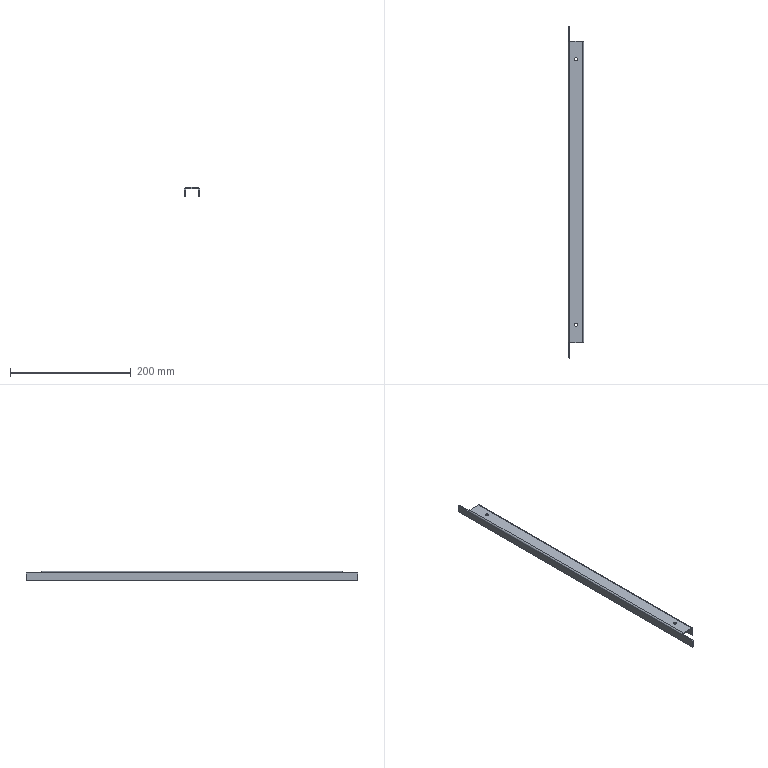Part | STEP file | Clamp Frame Weldment 2 | 1 solid | 22 faces | box 25 x 550 x 15 mm | volume 50877 mm3 | plane 14 | cylinder 8 | commonest cylinder face diameters 5.2 x4 1 x2 5 x2
STEP:
#1=CARTESIAN_POINT('',(-534.9,391.433,-2.));
#2=VERTEX_POINT('',#1);
#3=CARTESIAN_POINT('',(-540.1,391.433,-2.));
#4=VERTEX_POINT('',#3);
#5=CARTESIAN_POINT('',(-537.5,391.433,-2.));
#6=DIRECTION('',(0.,0.,-1.));
#7=DIRECTION('',(1.,0.,0.));
#8=AXIS2_PLACEMENT_3D('',#5,#6,#7);
#9=CIRCLE('',#8,2.6);
#10=EDGE_CURVE('',#2,#4,#9,.T.);
#11=ORIENTED_EDGE('',*,*,#10,.T.);
#12=CARTESIAN_POINT('',(-540.1,391.433,0.));
#13=VERTEX_POINT('',#12);
#14=CARTESIAN_POINT('',(-540.1,391.433,-10.));
#15=DIRECTION('',(0.,0.,1.));
#16=VECTOR('',#15,1000.);
#17=LINE('',#14,#16);
#18=EDGE_CURVE('',#4,#13,#17,.T.);
#19=ORIENTED_EDGE('',*,*,#18,.T.);
#20=CARTESIAN_POINT('',(-534.9,391.433,0.));
#21=VERTEX_POINT('',#20);
#22=CARTESIAN_POINT('',(-537.5,391.433,0.));
#23=DIRECTION('',(0.,0.,-1.));
#24=DIRECTION('',(1.,0.,0.));
#25=AXIS2_PLACEMENT_3D('',#22,#23,#24);
#26=CIRCLE('',#25,2.6);
#27=EDGE_CURVE('',#21,#13,#26,.T.);
#28=ORIENTED_EDGE('',*,*,#27,.F.);
#29=CARTESIAN_POINT('',(-534.9,391.433,-10.));
#30=DIRECTION('',(0.,0.,1.));
#31=VECTOR('',#30,1000.);
#32=LINE('',#29,#31);
#33=EDGE_CURVE('',#2,#21,#32,.T.);
#34=ORIENTED_EDGE('',*,*,#33,.F.);
#35=EDGE_LOOP('',(#11,#19,#28,#34));
#36=FACE_OUTER_BOUND('',#35,.T.);
#37=CARTESIAN_POINT('',(-537.5,391.433,-10.));
#38=DIRECTION('',(0.,0.,1.));
#39=DIRECTION('',(1.,0.,0.));
#40=AXIS2_PLACEMENT_3D('',#37,#38,#39);
#41=CYLINDRICAL_SURFACE('',#40,2.6);
#42=ADVANCED_FACE('',(#36),#41,.F.);
#43=CARTESIAN_POINT('',(-534.9,831.433,-2.));
#44=VERTEX_POINT('',#43);
#45=CARTESIAN_POINT('',(-540.1,831.433,-2.));
#46=VERTEX_POINT('',#45);
#47=CARTESIAN_POINT('',(-537.5,831.433,-2.));
#48=DIRECTION('',(0.,0.,-1.));
#49=DIRECTION('',(1.,0.,0.));
#50=AXIS2_PLACEMENT_3D('',#47,#48,#49);
#51=CIRCLE('',#50,2.6);
#52=EDGE_CURVE('',#44,#46,#51,.T.);
#53=ORIENTED_EDGE('',*,*,#52,.T.);
#54=CARTESIAN_POINT('',(-540.1,831.433,0.));
#55=VERTEX_POINT('',#54);
#56=CARTESIAN_POINT('',(-540.1,831.433,-10.));
#57=DIRECTION('',(0.,0.,1.));
#58=VECTOR('',#57,1000.);
#59=LINE('',#56,#58);
#60=EDGE_CURVE('',#46,#55,#59,.T.);
#61=ORIENTED_EDGE('',*,*,#60,.T.);
#62=CARTESIAN_POINT('',(-534.9,831.433,0.));
#63=VERTEX_POINT('',#62);
#64=CARTESIAN_POINT('',(-537.5,831.433,0.));
#65=DIRECTION('',(0.,0.,-1.));
#66=DIRECTION('',(1.,0.,0.));
#67=AXIS2_PLACEMENT_3D('',#64,#65,#66);
#68=CIRCLE('',#67,2.6);
#69=EDGE_CURVE('',#63,#55,#68,.T.);
#70=ORIENTED_EDGE('',*,*,#69,.F.);
#71=CARTESIAN_POINT('',(-534.9,831.433,-10.));
#72=DIRECTION('',(0.,0.,1.));
#73=VECTOR('',#72,1000.);
#74=LINE('',#71,#73);
#75=EDGE_CURVE('',#44,#63,#74,.T.);
#76=ORIENTED_EDGE('',*,*,#75,.F.);
#77=EDGE_LOOP('',(#53,#61,#70,#76));
#78=FACE_OUTER_BOUND('',#77,.T.);
#79=CARTESIAN_POINT('',(-537.5,831.433,-10.));
#80=DIRECTION('',(0.,0.,1.));
#81=DIRECTION('',(1.,0.,0.));
#82=AXIS2_PLACEMENT_3D('',#79,#80,#81);
#83=CYLINDRICAL_SURFACE('',#82,2.6);
#84=ADVANCED_FACE('',(#78),#83,.F.);
#85=CARTESIAN_POINT('',(-547.5,361.433,-2.));
#86=VERTEX_POINT('',#85);
#87=CARTESIAN_POINT('',(-527.5,361.433,-2.));
#88=VERTEX_POINT('',#87);
#89=CARTESIAN_POINT('',(0.,361.433,-2.));
#90=DIRECTION('',(1.,0.,0.));
#91=VECTOR('',#90,1000.);
#92=LINE('',#89,#91);
#93=EDGE_CURVE('',#86,#88,#92,.T.);
#94=ORIENTED_EDGE('',*,*,#93,.F.);
#95=CARTESIAN_POINT('',(-547.5,861.433,-2.));
#96=VERTEX_POINT('',#95);
#97=CARTESIAN_POINT('',(-547.5,0.,-2.));
#98=DIRECTION('',(0.,-1.,0.));
#99=VECTOR('',#98,1000.);
#100=LINE('',#97,#99);
#101=EDGE_CURVE('',#96,#86,#100,.T.);
#102=ORIENTED_EDGE('',*,*,#101,.F.);
#103=CARTESIAN_POINT('',(-527.5,861.433,-2.));
#104=VERTEX_POINT('',#103);
#105=CARTESIAN_POINT('',(0.,861.433,-2.));
#106=DIRECTION('',(-1.,0.,0.));
#107=VECTOR('',#106,1000.);
#108=LINE('',#105,#107);
#109=EDGE_CURVE('',#104,#96,#108,.T.);
#110=ORIENTED_EDGE('',*,*,#109,.F.);
#111=CARTESIAN_POINT('',(-527.5,0.,-2.));
#112=DIRECTION('',(0.,1.,0.));
#113=VECTOR('',#112,1000.);
#114=LINE('',#111,#113);
#115=EDGE_CURVE('',#88,#104,#114,.T.);
#116=ORIENTED_EDGE('',*,*,#115,.F.);
#117=EDGE_LOOP('',(#94,#102,#110,#116));
#118=FACE_OUTER_BOUND('',#117,.T.);
#119=ORIENTED_EDGE('',*,*,#10,.F.);
#120=CARTESIAN_POINT('',(-537.5,391.433,-2.));
#121=DIRECTION('',(0.,0.,-1.));
#122=DIRECTION('',(1.,0.,0.));
#123=AXIS2_PLACEMENT_3D('',#120,#121,#122);
#124=CIRCLE('',#123,2.6);
#125=EDGE_CURVE('',#4,#2,#124,.T.);
#126=ORIENTED_EDGE('',*,*,#125,.F.);
#127=EDGE_LOOP('',(#119,#126));
#128=FACE_BOUND('',#127,.T.);
#129=ORIENTED_EDGE('',*,*,#52,.F.);
#130=CARTESIAN_POINT('',(-537.5,831.433,-2.));
#131=DIRECTION('',(0.,0.,-1.));
#132=DIRECTION('',(1.,0.,0.));
#133=AXIS2_PLACEMENT_3D('',#130,#131,#132);
#134=CIRCLE('',#133,2.6);
#135=EDGE_CURVE('',#46,#44,#134,.T.);
#136=ORIENTED_EDGE('',*,*,#135,.F.);
#137=EDGE_LOOP('',(#129,#136));
#138=FACE_BOUND('',#137,.T.);
#139=CARTESIAN_POINT('',(0.,0.,-2.));
#140=DIRECTION('',(0.,0.,1.));
#141=DIRECTION('',(1.,0.,0.));
#142=AXIS2_PLACEMENT_3D('',#139,#140,#141);
#143=PLANE('',#142);
#144=ADVANCED_FACE('',(#118,#128,#138),#143,.F.);
#145=CARTESIAN_POINT('',(-527.,861.433,-2.5));
#146=VERTEX_POINT('',#145);
#147=CARTESIAN_POINT('',(-527.5,861.433,-2.5));
#148=DIRECTION('',(0.,-1.,0.));
#149=DIRECTION('',(0.,0.,-1.));
#150=AXIS2_PLACEMENT_3D('',#147,#148,#149);
#151=CIRCLE('',#150,0.5);
#152=EDGE_CURVE('',#146,#104,#151,.T.);
#153=ORIENTED_EDGE('',*,*,#152,.F.);
#154=CARTESIAN_POINT('',(-527.,361.433,-2.5));
#155=VERTEX_POINT('',#154);
#156=CARTESIAN_POINT('',(-527.,361.433,-2.5));
#157=DIRECTION('',(0.,1.,0.));
#158=VECTOR('',#157,1000.);
#159=LINE('',#156,#158);
#160=EDGE_CURVE('',#155,#146,#159,.T.);
#161=ORIENTED_EDGE('',*,*,#160,.F.);
#162=CARTESIAN_POINT('',(-527.5,361.433,-2.5));
#163=DIRECTION('',(0.,-1.,0.));
#164=DIRECTION('',(0.,0.,-1.));
#165=AXIS2_PLACEMENT_3D('',#162,#163,#164);
#166=CIRCLE('',#165,0.5);
#167=EDGE_CURVE('',#155,#88,#166,.T.);
#168=ORIENTED_EDGE('',*,*,#167,.T.);
#169=ORIENTED_EDGE('',*,*,#115,.T.);
#170=EDGE_LOOP('',(#153,#161,#168,#169));
#171=FACE_OUTER_BOUND('',#170,.T.);
#172=CARTESIAN_POINT('',(-527.5,361.433,-2.5));
#173=DIRECTION('',(0.,-1.,0.));
#174=DIRECTION('',(0.,0.,-1.));
#175=AXIS2_PLACEMENT_3D('',#172,#173,#174);
#176=CYLINDRICAL_SURFACE('',#175,0.5);
#177=ADVANCED_FACE('',(#171),#176,.F.);
#178=CARTESIAN_POINT('',(-527.5,361.433,0.));
#179=VERTEX_POINT('',#178);
#180=CARTESIAN_POINT('',(-547.5,361.433,0.));
#181=VERTEX_POINT('',#180);
#182=CARTESIAN_POINT('',(-525.,361.433,0.));
#183=DIRECTION('',(-1.,0.,0.));
#184=VECTOR('',#183,1000.);
#185=LINE('',#182,#184);
#186=EDGE_CURVE('',#179,#181,#185,.T.);
#187=ORIENTED_EDGE('',*,*,#186,.T.);
#188=CARTESIAN_POINT('',(-550.,361.433,-2.5));
#189=VERTEX_POINT('',#188);
#190=CARTESIAN_POINT('',(-547.5,361.433,-2.5));
#191=DIRECTION('',(0.,-1.,0.));
#192=DIRECTION('',(0.,0.,1.));
#193=AXIS2_PLACEMENT_3D('',#190,#191,#192);
#194=CIRCLE('',#193,2.5);
#195=EDGE_CURVE('',#181,#189,#194,.T.);
#196=ORIENTED_EDGE('',*,*,#195,.T.);
#197=CARTESIAN_POINT('',(-548.,361.433,-2.5));
#198=VERTEX_POINT('',#197);
#199=CARTESIAN_POINT('',(-547.5,361.433,-2.5));
#200=DIRECTION('',(1.,0.,0.));
#201=VECTOR('',#200,1000.);
#202=LINE('',#199,#201);
#203=EDGE_CURVE('',#189,#198,#202,.T.);
#204=ORIENTED_EDGE('',*,*,#203,.T.);
#205=CARTESIAN_POINT('',(-547.5,361.433,-2.5));
#206=DIRECTION('',(0.,1.,0.));
#207=DIRECTION('',(0.,0.,1.));
#208=AXIS2_PLACEMENT_3D('',#205,#206,#207);
#209=CIRCLE('',#208,0.5);
#210=EDGE_CURVE('',#198,#86,#209,.T.);
#211=ORIENTED_EDGE('',*,*,#210,.T.);
#212=ORIENTED_EDGE('',*,*,#93,.T.);
#213=ORIENTED_EDGE('',*,*,#167,.F.);
#214=CARTESIAN_POINT('',(-527.,361.433,-15.));
#215=VERTEX_POINT('',#214);
#216=CARTESIAN_POINT('',(-527.,361.433,0.));
#217=DIRECTION('',(0.,0.,1.));
#218=VECTOR('',#217,1000.);
#219=LINE('',#216,#218);
#220=EDGE_CURVE('',#215,#155,#219,.T.);
#221=ORIENTED_EDGE('',*,*,#220,.F.);
#222=CARTESIAN_POINT('',(-525.,361.433,-15.));
#223=VERTEX_POINT('',#222);
#224=CARTESIAN_POINT('',(-525.,361.433,-15.));
#225=DIRECTION('',(-1.,0.,0.));
#226=VECTOR('',#225,1000.);
#227=LINE('',#224,#226);
#228=EDGE_CURVE('',#223,#215,#227,.T.);
#229=ORIENTED_EDGE('',*,*,#228,.F.);
#230=CARTESIAN_POINT('',(-525.,361.433,-2.5));
#231=VERTEX_POINT('',#230);
#232=CARTESIAN_POINT('',(-525.,361.433,-15.));
#233=DIRECTION('',(0.,0.,1.));
#234=VECTOR('',#233,1000.);
#235=LINE('',#232,#234);
#236=EDGE_CURVE('',#223,#231,#235,.T.);
#237=ORIENTED_EDGE('',*,*,#236,.T.);
#238=CARTESIAN_POINT('',(-527.5,361.433,-2.5));
#239=DIRECTION('',(0.,1.,0.));
#240=DIRECTION('',(0.,0.,-1.));
#241=AXIS2_PLACEMENT_3D('',#238,#239,#240);
#242=CIRCLE('',#241,2.5);
#243=EDGE_CURVE('',#179,#231,#242,.T.);
#244=ORIENTED_EDGE('',*,*,#243,.F.);
#245=EDGE_LOOP('',(#187,#196,#204,#211,#212,#213,#221,#229,#237,#244));
#246=FACE_OUTER_BOUND('',#245,.T.);
#247=CARTESIAN_POINT('',(-525.,361.433,-2.));
#248=DIRECTION('',(0.,-1.,0.));
#249=DIRECTION('',(1.,0.,0.));
#250=AXIS2_PLACEMENT_3D('',#247,#248,#249);
#251=PLANE('',#250);
#252=ADVANCED_FACE('',(#246),#251,.T.);
#253=ORIENTED_EDGE('',*,*,#210,.F.);
#254=CARTESIAN_POINT('',(-548.,861.433,-2.5));
#255=VERTEX_POINT('',#254);
#256=CARTESIAN_POINT('',(-548.,861.433,-2.5));
#257=DIRECTION('',(0.,-1.,0.));
#258=VECTOR('',#257,1000.);
#259=LINE('',#256,#258);
#260=EDGE_CURVE('',#255,#198,#259,.T.);
#261=ORIENTED_EDGE('',*,*,#260,.F.);
#262=CARTESIAN_POINT('',(-547.5,861.433,-2.5));
#263=DIRECTION('',(0.,1.,0.));
#264=DIRECTION('',(0.,0.,1.));
#265=AXIS2_PLACEMENT_3D('',#262,#263,#264);
#266=CIRCLE('',#265,0.5);
#267=EDGE_CURVE('',#255,#96,#266,.T.);
#268=ORIENTED_EDGE('',*,*,#267,.T.);
#269=ORIENTED_EDGE('',*,*,#101,.T.);
#270=EDGE_LOOP('',(#253,#261,#268,#269));
#271=FACE_OUTER_BOUND('',#270,.T.);
#272=CARTESIAN_POINT('',(-547.5,861.433,-2.5));
#273=DIRECTION('',(0.,1.,0.));
#274=DIRECTION('',(0.,0.,1.));
#275=AXIS2_PLACEMENT_3D('',#272,#273,#274);
#276=CYLINDRICAL_SURFACE('',#275,0.5);
#277=ADVANCED_FACE('',(#271),#276,.F.);
#278=ORIENTED_EDGE('',*,*,#109,.T.);
#279=ORIENTED_EDGE('',*,*,#267,.F.);
#280=CARTESIAN_POINT('',(-550.,861.433,-2.5));
#281=VERTEX_POINT('',#280);
#282=CARTESIAN_POINT('',(-547.5,861.433,-2.5));
#283=DIRECTION('',(1.,0.,0.));
#284=VECTOR('',#283,1000.);
#285=LINE('',#282,#284);
#286=EDGE_CURVE('',#281,#255,#285,.T.);
#287=ORIENTED_EDGE('',*,*,#286,.F.);
#288=CARTESIAN_POINT('',(-547.5,861.433,0.));
#289=VERTEX_POINT('',#288);
#290=CARTESIAN_POINT('',(-547.5,861.433,-2.5));
#291=DIRECTION('',(0.,-1.,0.));
#292=DIRECTION('',(0.,0.,1.));
#293=AXIS2_PLACEMENT_3D('',#290,#291,#292);
#294=CIRCLE('',#293,2.5);
#295=EDGE_CURVE('',#289,#281,#294,.T.);
#296=ORIENTED_EDGE('',*,*,#295,.F.);
#297=CARTESIAN_POINT('',(-527.5,861.433,0.));
#298=VERTEX_POINT('',#297);
#299=CARTESIAN_POINT('',(-525.,861.433,0.));
#300=DIRECTION('',(1.,0.,0.));
#301=VECTOR('',#300,1000.);
#302=LINE('',#299,#301);
#303=EDGE_CURVE('',#289,#298,#302,.T.);
#304=ORIENTED_EDGE('',*,*,#303,.T.);
#305=CARTESIAN_POINT('',(-525.,861.433,-2.5));
#306=VERTEX_POINT('',#305);
#307=CARTESIAN_POINT('',(-527.5,861.433,-2.5));
#308=DIRECTION('',(0.,1.,0.));
#309=DIRECTION('',(0.,0.,-1.));
#310=AXIS2_PLACEMENT_3D('',#307,#308,#309);
#311=CIRCLE('',#310,2.5);
#312=EDGE_CURVE('',#298,#306,#311,.T.);
#313=ORIENTED_EDGE('',*,*,#312,.T.);
#314=CARTESIAN_POINT('',(-525.,861.433,-15.));
#315=VERTEX_POINT('',#314);
#316=CARTESIAN_POINT('',(-525.,861.433,-2.));
#317=DIRECTION('',(0.,0.,-1.));
#318=VECTOR('',#317,1000.);
#319=LINE('',#316,#318);
#320=EDGE_CURVE('',#306,#315,#319,.T.);
#321=ORIENTED_EDGE('',*,*,#320,.T.);
#322=CARTESIAN_POINT('',(-527.,861.433,-15.));
#323=VERTEX_POINT('',#322);
#324=CARTESIAN_POINT('',(-525.,861.433,-15.));
#325=DIRECTION('',(1.,0.,0.));
#326=VECTOR('',#325,1000.);
#327=LINE('',#324,#326);
#328=EDGE_CURVE('',#323,#315,#327,.T.);
#329=ORIENTED_EDGE('',*,*,#328,.F.);
#330=CARTESIAN_POINT('',(-527.,861.433,0.));
#331=DIRECTION('',(0.,0.,-1.));
#332=VECTOR('',#331,1000.);
#333=LINE('',#330,#332);
#334=EDGE_CURVE('',#146,#323,#333,.T.);
#335=ORIENTED_EDGE('',*,*,#334,.F.);
#336=ORIENTED_EDGE('',*,*,#152,.T.);
#337=EDGE_LOOP('',(#278,#279,#287,#296,#304,#313,#321,#329,#335,#336));
#338=FACE_OUTER_BOUND('',#337,.T.);
#339=CARTESIAN_POINT('',(-525.,861.433,-2.));
#340=DIRECTION('',(0.,1.,0.));
#341=DIRECTION('',(0.,0.,1.));
#342=AXIS2_PLACEMENT_3D('',#339,#340,#341);
#343=PLANE('',#342);
#344=ADVANCED_FACE('',(#338),#343,.T.);
#345=ORIENTED_EDGE('',*,*,#18,.F.);
#346=ORIENTED_EDGE('',*,*,#125,.T.);
#347=ORIENTED_EDGE('',*,*,#33,.T.);
#348=CARTESIAN_POINT('',(-537.5,391.433,0.));
#349=DIRECTION('',(0.,0.,-1.));
#350=DIRECTION('',(1.,0.,0.));
#351=AXIS2_PLACEMENT_3D('',#348,#349,#350);
#352=CIRCLE('',#351,2.6);
#353=EDGE_CURVE('',#13,#21,#352,.T.);
#354=ORIENTED_EDGE('',*,*,#353,.F.);
#355=EDGE_LOOP('',(#345,#346,#347,#354));
#356=FACE_OUTER_BOUND('',#355,.T.);
#357=CARTESIAN_POINT('',(-537.5,391.433,-10.));
#358=DIRECTION('',(0.,0.,1.));
#359=DIRECTION('',(1.,0.,0.));
#360=AXIS2_PLACEMENT_3D('',#357,#358,#359);
#361=CYLINDRICAL_SURFACE('',#360,2.6);
#362=ADVANCED_FACE('',(#356),#361,.F.);
#363=ORIENTED_EDGE('',*,*,#60,.F.);
#364=ORIENTED_EDGE('',*,*,#135,.T.);
#365=ORIENTED_EDGE('',*,*,#75,.T.);
#366=CARTESIAN_POINT('',(-537.5,831.433,0.));
#367=DIRECTION('',(0.,0.,-1.));
#368=DIRECTION('',(1.,0.,0.));
#369=AXIS2_PLACEMENT_3D('',#366,#367,#368);
#370=CIRCLE('',#369,2.6);
#371=EDGE_CURVE('',#55,#63,#370,.T.);
#372=ORIENTED_EDGE('',*,*,#371,.F.);
#373=EDGE_LOOP('',(#363,#364,#365,#372));
#374=FACE_OUTER_BOUND('',#373,.T.);
#375=CARTESIAN_POINT('',(-537.5,831.433,-10.));
#376=DIRECTION('',(0.,0.,1.));
#377=DIRECTION('',(1.,0.,0.));
#378=AXIS2_PLACEMENT_3D('',#375,#376,#377);
#379=CYLINDRICAL_SURFACE('',#378,2.6);
#380=ADVANCED_FACE('',(#374),#379,.F.);
#381=ORIENTED_EDGE('',*,*,#334,.T.);
#382=CARTESIAN_POINT('',(-527.,0.,-15.));
#383=DIRECTION('',(0.,-1.,0.));
#384=VECTOR('',#383,1000.);
#385=LINE('',#382,#384);
#386=EDGE_CURVE('',#323,#215,#385,.T.);
#387=ORIENTED_EDGE('',*,*,#386,.T.);
#388=ORIENTED_EDGE('',*,*,#220,.T.);
#389=ORIENTED_EDGE('',*,*,#160,.T.);
#390=EDGE_LOOP('',(#381,#387,#388,#389));
#391=FACE_OUTER_BOUND('',#390,.T.);
#392=CARTESIAN_POINT('',(-527.,0.,0.));
#393=DIRECTION('',(-1.,0.,0.));
#394=DIRECTION('',(0.,0.,1.));
#395=AXIS2_PLACEMENT_3D('',#392,#393,#394);
#396=PLANE('',#395);
#397=ADVANCED_FACE('',(#391),#396,.T.);
#398=ORIENTED_EDGE('',*,*,#303,.F.);
#399=CARTESIAN_POINT('',(-547.5,0.,0.));
#400=DIRECTION('',(0.,-1.,0.));
#401=VECTOR('',#400,1000.);
#402=LINE('',#399,#401);
#403=EDGE_CURVE('',#289,#181,#402,.T.);
#404=ORIENTED_EDGE('',*,*,#403,.T.);
#405=ORIENTED_EDGE('',*,*,#186,.F.);
#406=CARTESIAN_POINT('',(-527.5,0.,0.));
#407=DIRECTION('',(0.,1.,0.));
#408=VECTOR('',#407,1000.);
#409=LINE('',#406,#408);
#410=EDGE_CURVE('',#179,#298,#409,.T.);
#411=ORIENTED_EDGE('',*,*,#410,.T.);
#412=EDGE_LOOP('',(#398,#404,#405,#411));
#413=FACE_OUTER_BOUND('',#412,.T.);
#414=ORIENTED_EDGE('',*,*,#27,.T.);
#415=ORIENTED_EDGE('',*,*,#353,.T.);
#416=EDGE_LOOP('',(#414,#415));
#417=FACE_BOUND('',#416,.T.);
#418=ORIENTED_EDGE('',*,*,#69,.T.);
#419=ORIENTED_EDGE('',*,*,#371,.T.);
#420=EDGE_LOOP('',(#418,#419));
#421=FACE_BOUND('',#420,.T.);
#422=CARTESIAN_POINT('',(0.,0.,0.));
#423=DIRECTION('',(0.,0.,1.));
#424=DIRECTION('',(1.,0.,0.));
#425=AXIS2_PLACEMENT_3D('',#422,#423,#424);
#426=PLANE('',#425);
#427=ADVANCED_FACE('',(#413,#417,#421),#426,.T.);
#428=CARTESIAN_POINT('',(-548.,336.433,-2.5));
#429=VERTEX_POINT('',#428);
#430=CARTESIAN_POINT('',(-548.,0.,-2.5));
#431=DIRECTION('',(0.,1.,0.));
#432=VECTOR('',#431,1000.);
#433=LINE('',#430,#432);
#434=EDGE_CURVE('',#429,#198,#433,.T.);
#435=ORIENTED_EDGE('',*,*,#434,.F.);
#436=CARTESIAN_POINT('',(-548.,336.433,-15.));
#437=VERTEX_POINT('',#436);
#438=CARTESIAN_POINT('',(-548.,336.433,0.));
#439=DIRECTION('',(0.,0.,1.));
#440=VECTOR('',#439,1000.);
#441=LINE('',#438,#440);
#442=EDGE_CURVE('',#437,#429,#441,.T.);
#443=ORIENTED_EDGE('',*,*,#442,.F.);
#444=CARTESIAN_POINT('',(-548.,886.433,-15.));
#445=VERTEX_POINT('',#444);
#446=CARTESIAN_POINT('',(-548.,0.,-15.));
#447=DIRECTION('',(0.,-1.,0.));
#448=VECTOR('',#447,1000.);
#449=LINE('',#446,#448);
#450=EDGE_CURVE('',#445,#437,#449,.T.);
#451=ORIENTED_EDGE('',*,*,#450,.F.);
#452=CARTESIAN_POINT('',(-548.,886.433,-2.5));
#453=VERTEX_POINT('',#452);
#454=CARTESIAN_POINT('',(-548.,886.433,0.));
#455=DIRECTION('',(0.,0.,-1.));
#456=VECTOR('',#455,1000.);
#457=LINE('',#454,#456);
#458=EDGE_CURVE('',#453,#445,#457,.T.);
#459=ORIENTED_EDGE('',*,*,#458,.F.);
#460=CARTESIAN_POINT('',(-548.,0.,-2.5));
#461=DIRECTION('',(0.,1.,0.));
#462=VECTOR('',#461,1000.);
#463=LINE('',#460,#462);
#464=EDGE_CURVE('',#255,#453,#463,.T.);
#465=ORIENTED_EDGE('',*,*,#464,.F.);
#466=ORIENTED_EDGE('',*,*,#260,.T.);
#467=EDGE_LOOP('',(#435,#443,#451,#459,#465,#466));
#468=FACE_OUTER_BOUND('',#467,.T.);
#469=CARTESIAN_POINT('',(-548.,0.,0.));
#470=DIRECTION('',(-1.,0.,0.));
#471=DIRECTION('',(0.,-1.,0.));
#472=AXIS2_PLACEMENT_3D('',#469,#470,#471);
#473=PLANE('',#472);
#474=ADVANCED_FACE('',(#468),#473,.F.);
#475=CARTESIAN_POINT('',(-525.,861.433,-15.));
#476=DIRECTION('',(0.,-1.,0.));
#477=VECTOR('',#476,1000.);
#478=LINE('',#475,#477);
#479=EDGE_CURVE('',#315,#223,#478,.T.);
#480=ORIENTED_EDGE('',*,*,#479,.T.);
#481=ORIENTED_EDGE('',*,*,#228,.T.);
#482=ORIENTED_EDGE('',*,*,#386,.F.);
#483=ORIENTED_EDGE('',*,*,#328,.T.);
#484=EDGE_LOOP('',(#480,#481,#482,#483));
#485=FACE_OUTER_BOUND('',#484,.T.);
#486=CARTESIAN_POINT('',(-525.,861.433,-15.));
#487=DIRECTION('',(0.,0.,-1.));
#488=DIRECTION('',(-1.,0.,0.));
#489=AXIS2_PLACEMENT_3D('',#486,#487,#488);
#490=PLANE('',#489);
#491=ADVANCED_FACE('',(#485),#490,.T.);
#492=CARTESIAN_POINT('',(-550.,861.433,-2.5));
#493=DIRECTION('',(0.,-1.,0.));
#494=VECTOR('',#493,1000.);
#495=LINE('',#492,#494);
#496=EDGE_CURVE('',#281,#189,#495,.T.);
#497=ORIENTED_EDGE('',*,*,#496,.T.);
#498=ORIENTED_EDGE('',*,*,#195,.F.);
#499=ORIENTED_EDGE('',*,*,#403,.F.);
#500=ORIENTED_EDGE('',*,*,#295,.T.);
#501=EDGE_LOOP('',(#497,#498,#499,#500));
#502=FACE_OUTER_BOUND('',#501,.T.);
#503=CARTESIAN_POINT('',(-547.5,861.433,-2.5));
#504=DIRECTION('',(0.,1.,0.));
#505=DIRECTION('',(0.,0.,1.));
#506=AXIS2_PLACEMENT_3D('',#503,#504,#505);
#507=CYLINDRICAL_SURFACE('',#506,2.5);
#508=ADVANCED_FACE('',(#502),#507,.T.);
#509=CARTESIAN_POINT('',(-550.,336.433,-2.5));
#510=VERTEX_POINT('',#509);
#511=CARTESIAN_POINT('',(-550.,336.433,-2.5));
#512=DIRECTION('',(0.,1.,0.));
#513=VECTOR('',#512,1000.);
#514=LINE('',#511,#513);
#515=EDGE_CURVE('',#510,#189,#514,.T.);
#516=ORIENTED_EDGE('',*,*,#515,.F.);
#517=CARTESIAN_POINT('',(-548.,336.433,-2.5));
#518=DIRECTION('',(-1.,0.,0.));
#519=VECTOR('',#518,1000.);
#520=LINE('',#517,#519);
#521=EDGE_CURVE('',#429,#510,#520,.T.);
#522=ORIENTED_EDGE('',*,*,#521,.F.);
#523=ORIENTED_EDGE('',*,*,#434,.T.);
#524=ORIENTED_EDGE('',*,*,#203,.F.);
#525=EDGE_LOOP('',(#516,#522,#523,#524));
#526=FACE_OUTER_BOUND('',#525,.T.);
#527=CARTESIAN_POINT('',(-548.,336.433,-2.5));
#528=DIRECTION('',(0.,0.,-1.));
#529=DIRECTION('',(-1.,0.,0.));
#530=AXIS2_PLACEMENT_3D('',#527,#528,#529);
#531=PLANE('',#530);
#532=ADVANCED_FACE('',(#526),#531,.F.);
#533=CARTESIAN_POINT('',(-525.,361.433,-2.5));
#534=DIRECTION('',(0.,1.,0.));
#535=VECTOR('',#534,1000.);
#536=LINE('',#533,#535);
#537=EDGE_CURVE('',#231,#306,#536,.T.);
#538=ORIENTED_EDGE('',*,*,#537,.T.);
#539=ORIENTED_EDGE('',*,*,#312,.F.);
#540=ORIENTED_EDGE('',*,*,#410,.F.);
#541=ORIENTED_EDGE('',*,*,#243,.T.);
#542=EDGE_LOOP('',(#538,#539,#540,#541));
#543=FACE_OUTER_BOUND('',#542,.T.);
#544=CARTESIAN_POINT('',(-527.5,361.433,-2.5));
#545=DIRECTION('',(0.,-1.,0.));
#546=DIRECTION('',(0.,0.,-1.));
#547=AXIS2_PLACEMENT_3D('',#544,#545,#546);
#548=CYLINDRICAL_SURFACE('',#547,2.5);
#549=ADVANCED_FACE('',(#543),#548,.T.);
#550=ORIENTED_EDGE('',*,*,#521,.T.);
#551=CARTESIAN_POINT('',(-550.,336.433,-15.));
#552=VERTEX_POINT('',#551);
#553=CARTESIAN_POINT('',(-550.,336.433,0.));
#554=DIRECTION('',(0.,0.,-1.));
#555=VECTOR('',#554,1000.);
#556=LINE('',#553,#555);
#557=EDGE_CURVE('',#510,#552,#556,.T.);
#558=ORIENTED_EDGE('',*,*,#557,.T.);
#559=CARTESIAN_POINT('',(0.,336.433,-15.));
#560=DIRECTION('',(1.,0.,0.));
#561=VECTOR('',#560,1000.);
#562=LINE('',#559,#561);
#563=EDGE_CURVE('',#552,#437,#562,.T.);
#564=ORIENTED_EDGE('',*,*,#563,.T.);
#565=ORIENTED_EDGE('',*,*,#442,.T.);
#566=EDGE_LOOP('',(#550,#558,#564,#565));
#567=FACE_OUTER_BOUND('',#566,.T.);
#568=CARTESIAN_POINT('',(0.,336.433,0.));
#569=DIRECTION('',(0.,-1.,0.));
#570=DIRECTION('',(0.,0.,-1.));
#571=AXIS2_PLACEMENT_3D('',#568,#569,#570);
#572=PLANE('',#571);
#573=ADVANCED_FACE('',(#567),#572,.T.);
#574=CARTESIAN_POINT('',(-550.,886.433,-15.));
#575=VERTEX_POINT('',#574);
#576=CARTESIAN_POINT('',(-550.,861.433,-15.));
#577=DIRECTION('',(0.,1.,0.));
#578=VECTOR('',#577,1000.);
#579=LINE('',#576,#578);
#580=EDGE_CURVE('',#552,#575,#579,.T.);
#581=ORIENTED_EDGE('',*,*,#580,.T.);
#582=CARTESIAN_POINT('',(-550.,886.433,-15.));
#583=DIRECTION('',(1.,0.,0.));
#584=VECTOR('',#583,1000.);
#585=LINE('',#582,#584);
#586=EDGE_CURVE('',#575,#445,#585,.T.);
#587=ORIENTED_EDGE('',*,*,#586,.T.);
#588=ORIENTED_EDGE('',*,*,#450,.T.);
#589=ORIENTED_EDGE('',*,*,#563,.F.);
#590=EDGE_LOOP('',(#581,#587,#588,#589));
#591=FACE_OUTER_BOUND('',#590,.T.);
#592=CARTESIAN_POINT('',(-550.,861.433,-15.));
#593=DIRECTION('',(0.,0.,-1.));
#594=DIRECTION('',(-1.,0.,0.));
#595=AXIS2_PLACEMENT_3D('',#592,#593,#594);
#596=PLANE('',#595);
#597=ADVANCED_FACE('',(#591),#596,.T.);
#598=CARTESIAN_POINT('',(-550.,886.433,-2.5));
#599=VERTEX_POINT('',#598);
#600=CARTESIAN_POINT('',(0.,886.433,-2.5));
#601=DIRECTION('',(1.,0.,0.));
#602=VECTOR('',#601,1000.);
#603=LINE('',#600,#602);
#604=EDGE_CURVE('',#599,#453,#603,.T.);
#605=ORIENTED_EDGE('',*,*,#604,.T.);
#606=ORIENTED_EDGE('',*,*,#458,.T.);
#607=ORIENTED_EDGE('',*,*,#586,.F.);
#608=CARTESIAN_POINT('',(-550.,886.433,0.));
#609=DIRECTION('',(0.,0.,1.));
#610=VECTOR('',#609,1000.);
#611=LINE('',#608,#610);
#612=EDGE_CURVE('',#575,#599,#611,.T.);
#613=ORIENTED_EDGE('',*,*,#612,.T.);
#614=EDGE_LOOP('',(#605,#606,#607,#613));
#615=FACE_OUTER_BOUND('',#614,.T.);
#616=CARTESIAN_POINT('',(0.,886.433,0.));
#617=DIRECTION('',(0.,1.,0.));
#618=DIRECTION('',(0.,0.,1.));
#619=AXIS2_PLACEMENT_3D('',#616,#617,#618);
#620=PLANE('',#619);
#621=ADVANCED_FACE('',(#615),#620,.T.);
#622=ORIENTED_EDGE('',*,*,#464,.T.);
#623=ORIENTED_EDGE('',*,*,#604,.F.);
#624=CARTESIAN_POINT('',(-550.,886.433,-2.5));
#625=DIRECTION('',(0.,1.,0.));
#626=VECTOR('',#625,1000.);
#627=LINE('',#624,#626);
#628=EDGE_CURVE('',#281,#599,#627,.T.);
#629=ORIENTED_EDGE('',*,*,#628,.F.);
#630=ORIENTED_EDGE('',*,*,#286,.T.);
#631=EDGE_LOOP('',(#622,#623,#629,#630));
#632=FACE_OUTER_BOUND('',#631,.T.);
#633=CARTESIAN_POINT('',(-550.,886.433,-2.5));
#634=DIRECTION('',(0.,0.,-1.));
#635=DIRECTION('',(-1.,0.,0.));
#636=AXIS2_PLACEMENT_3D('',#633,#634,#635);
#637=PLANE('',#636);
#638=ADVANCED_FACE('',(#632),#637,.F.);
#639=ORIENTED_EDGE('',*,*,#236,.F.);
#640=ORIENTED_EDGE('',*,*,#479,.F.);
#641=ORIENTED_EDGE('',*,*,#320,.F.);
#642=ORIENTED_EDGE('',*,*,#537,.F.);
#643=EDGE_LOOP('',(#639,#640,#641,#642));
#644=FACE_OUTER_BOUND('',#643,.T.);
#645=CARTESIAN_POINT('',(-525.,0.,0.));
#646=DIRECTION('',(-1.,0.,0.));
#647=DIRECTION('',(0.,0.,1.));
#648=AXIS2_PLACEMENT_3D('',#645,#646,#647);
#649=PLANE('',#648);
#650=ADVANCED_FACE('',(#644),#649,.F.);
#651=ORIENTED_EDGE('',*,*,#628,.T.);
#652=ORIENTED_EDGE('',*,*,#612,.F.);
#653=ORIENTED_EDGE('',*,*,#580,.F.);
#654=ORIENTED_EDGE('',*,*,#557,.F.);
#655=ORIENTED_EDGE('',*,*,#515,.T.);
#656=ORIENTED_EDGE('',*,*,#496,.F.);
#657=EDGE_LOOP('',(#651,#652,#653,#654,#655,#656));
#658=FACE_OUTER_BOUND('',#657,.T.);
#659=CARTESIAN_POINT('',(-550.,0.,0.));
#660=DIRECTION('',(-1.,0.,0.));
#661=DIRECTION('',(0.,-1.,0.));
#662=AXIS2_PLACEMENT_3D('',#659,#660,#661);
#663=PLANE('',#662);
#664=ADVANCED_FACE('',(#658),#663,.T.);
#665=CLOSED_SHELL('',(#42,#84,#144,#177,#252,#277,#344,#362,#380,#397,#427,#474,#491,#508,#532,#549,#573,#597,#621,#638,#650,#664));
#666=MANIFOLD_SOLID_BREP('',#665);
#667=CARTESIAN_POINT('',(0.,0.,0.));
#668=DIRECTION('',(0.,0.,1.));
#669=DIRECTION('',(1.,0.,0.));
#670=AXIS2_PLACEMENT_3D('',#667,#668,#669);
#671=(LENGTH_UNIT()NAMED_UNIT(*)SI_UNIT(.MILLI.,.METRE.));
#672=UNCERTAINTY_MEASURE_WITH_UNIT(LENGTH_MEASURE(0.00001),#671,'','');
#673=(NAMED_UNIT(*)PLANE_ANGLE_UNIT()SI_UNIT($,.RADIAN.));
#674=(NAMED_UNIT(*)SI_UNIT($,.STERADIAN.)SOLID_ANGLE_UNIT());
#675=(GEOMETRIC_REPRESENTATION_CONTEXT(3)GLOBAL_UNCERTAINTY_ASSIGNED_CONTEXT((#672))GLOBAL_UNIT_ASSIGNED_CONTEXT((#671,#673,#674))REPRESENTATION_CONTEXT('',''));
#676=ADVANCED_BREP_SHAPE_REPRESENTATION('',(#666,#670),#675);